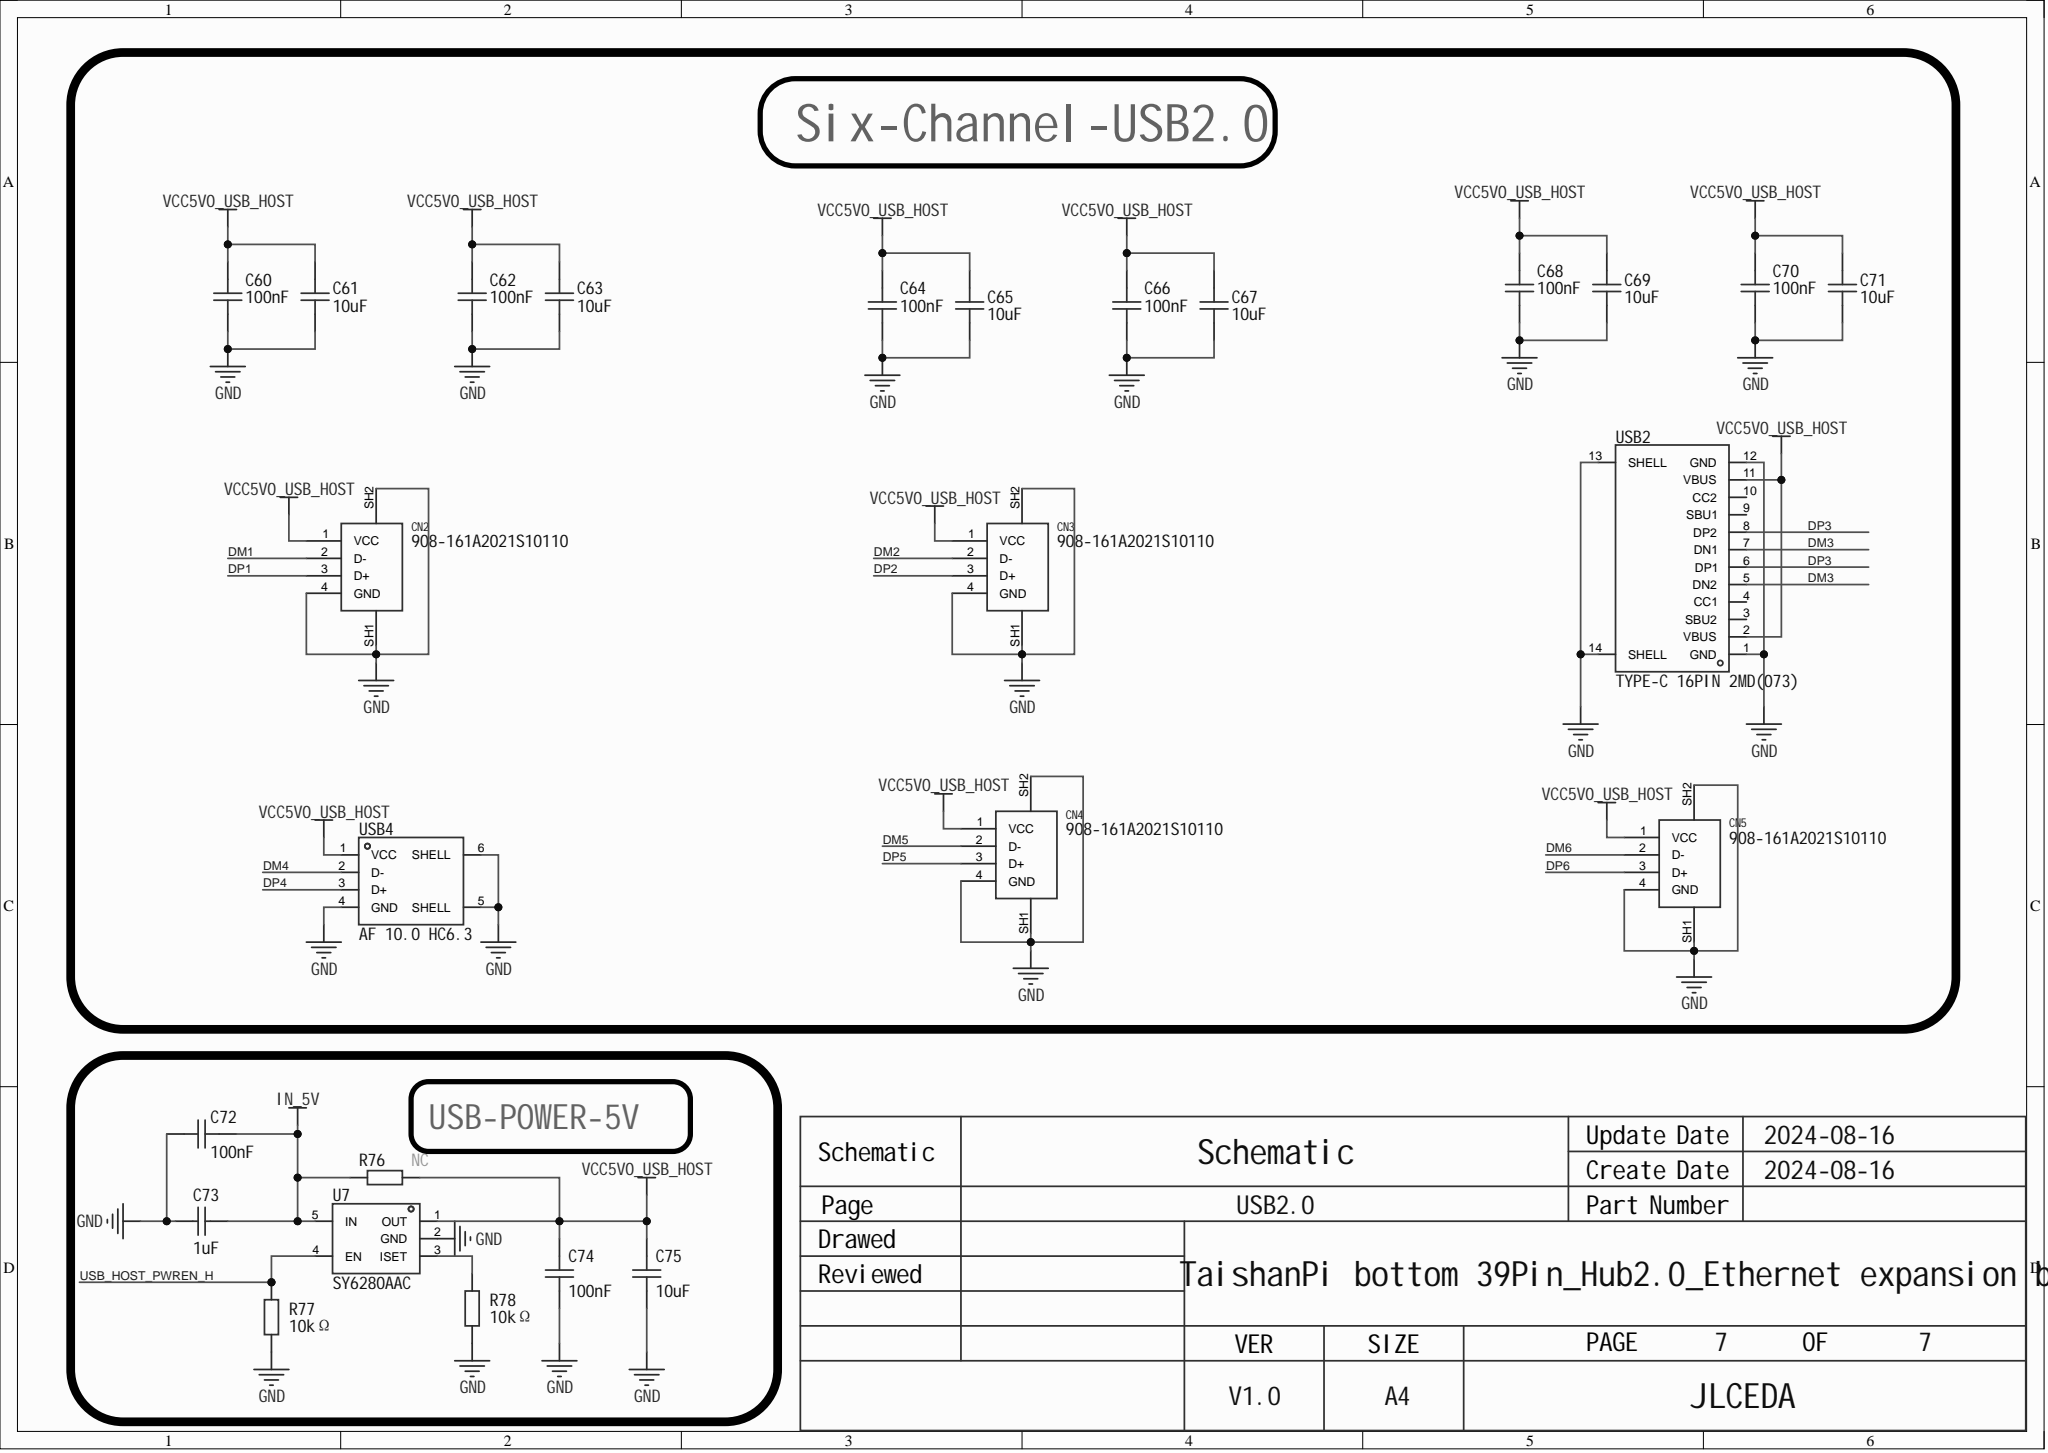Circuit board | Altium Designer | 209 parts | 149 nets | one sheet of the schematic
Parts on this sheet (reference | value | footprint):
C60 | 100nF | R0402
C61 | 10uF | R0402
C62 | 100nF | r0603
C63 | 10uF | r0603
C64 | 100nF | r0603
C65 | 10uF | r0603
C66 | 100nF | r0603
C67 | 10uF | r0603
C68 | 100nF | r0603
C69 | 10uF | r0603
C70 | 100nF | r0603
C71 | 10uF | r0603
C72 | 100nF | C0603
C73 | 1uF | C0603
C74 | 100nF | C0603
C75 | 10uF | C0603
CN2 | 908-161A2021S10110 | USB-A-SMD_AF-SMT-SHORT
CN3 | 908-161A2021S10110 | USB-A-SMD_AF-SMT-SHORT
CN4 | 908-161A2021S10110 | USB-A-SMD_AF-SMT-SHORT
CN5 | 908-161A2021S10110 | USB-A-SMD_AF-SMT-SHORT
R76 | NC | R0805
R77 | 10kΩ | R0402
R78 | 10kΩ | R0402
U7 | SY6280AAC | SOT-23-5_L3.0-W1.7-P0.95-LS2.8-BL
USB2 | TYPE-C 16PIN 2MD(073) | USB-C-SMD_TYPE-C-6PIN-2MD-073
USB4 | AF 10.0 HC6.3 | USB-A-TH_AF-10.0-HC6.3
Nets of these parts (net: part-pin ...):
VCC5V0_USB_HOST: C60-2 C61-2 C62-2 C63-2 C64-2 C65-2 C66-2 C67-2 C68-2 C69-2 C70-2 C71-2 C74-2 C75-2 CN2-1 CN3-1 CN4-1 CN5-1 R76-2 U7-1 USB2-2 USB2-11 USB4-1
NetR78_2: R78-2 U7-3
IN_5V: C72-1 C73-2 R76-1 U7-5
GPIO0_A5: R77-2 U7-4
GND: C60-1 C61-1 C62-1 C63-1 C64-1 C65-1 C66-1 C67-1 C68-1 C69-1 C70-1 C71-1 C72-2 C73-1 C74-1 C75-1 CN2-4 CN2-SH1 CN2-SH2 CN3-4 CN3-SH1 CN3-SH2 CN4-4 CN4-SH1 CN4-SH2 CN5-4 CN5-SH1 CN5-SH2 R77-1 R78-1 U7-2 USB2-1 USB2-12 USB2-13 USB2-14 USB4-4 USB4-5 USB4-6
DP6: CN5-3
DP5: CN4-3
DP4: USB4-3
DP3: USB2-6 USB2-8
DP2: CN3-3
DP1: CN2-3
DM6: CN5-2
DM5: CN4-2
DM4: USB4-2
DM3: USB2-5 USB2-7
DM2: CN3-2
DM1: CN2-2